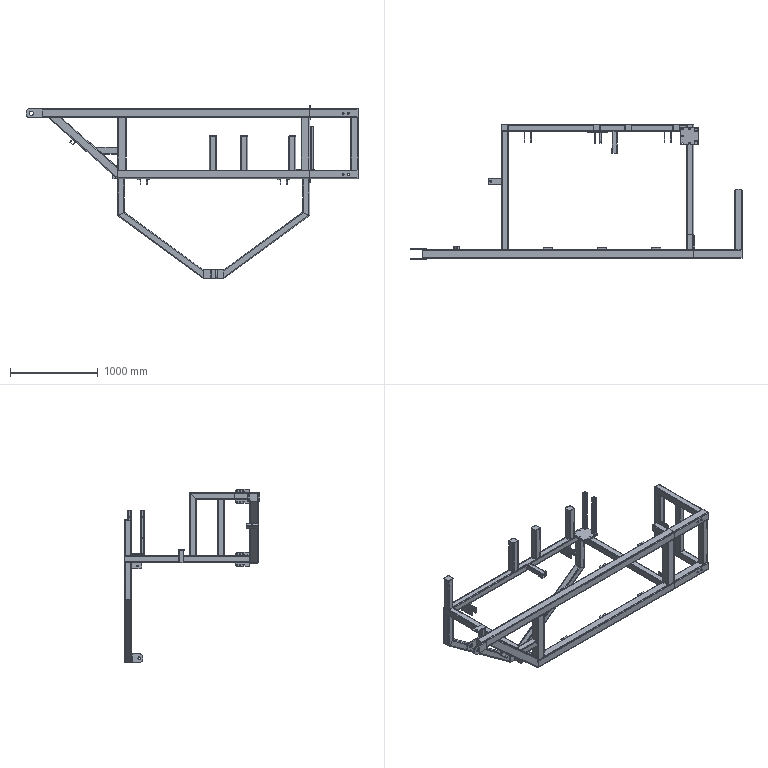Part | STEP file | 01_GLOWNA_RAMAV11_Default<Obrobiona> | 62 solids | 960 faces | box 3794 x 1545 x 1980 mm | volume 40557701 mm3 | plane 516 | cylinder 444 | commonest cylinder face diameters 20 x144 10 x132 16 x33 21 x26 14 x24 12 x16